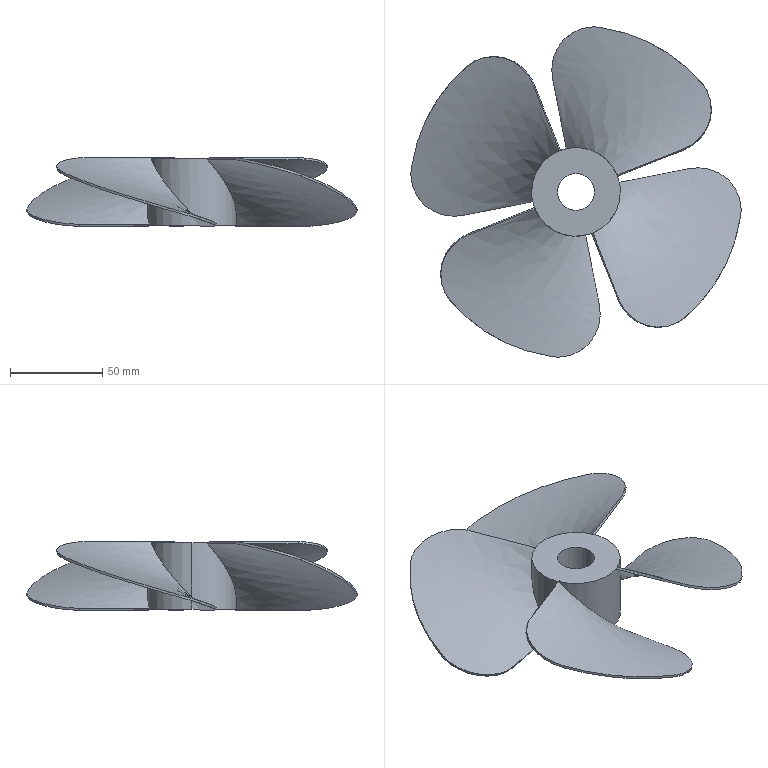Part | SolidWorks | features ICE 2, 3DProfileFeature 1, BaseBody 1, HoleWzd 1, Scale 1 | 1 solid | 53 faces | box 178.664 x 178.664 x 37.098 mm | volume 66695 mm3 | spline 40 | cylinder 11 | plane 2 | commonest cylinder face diameters 48 x7 5 x2 20 x2